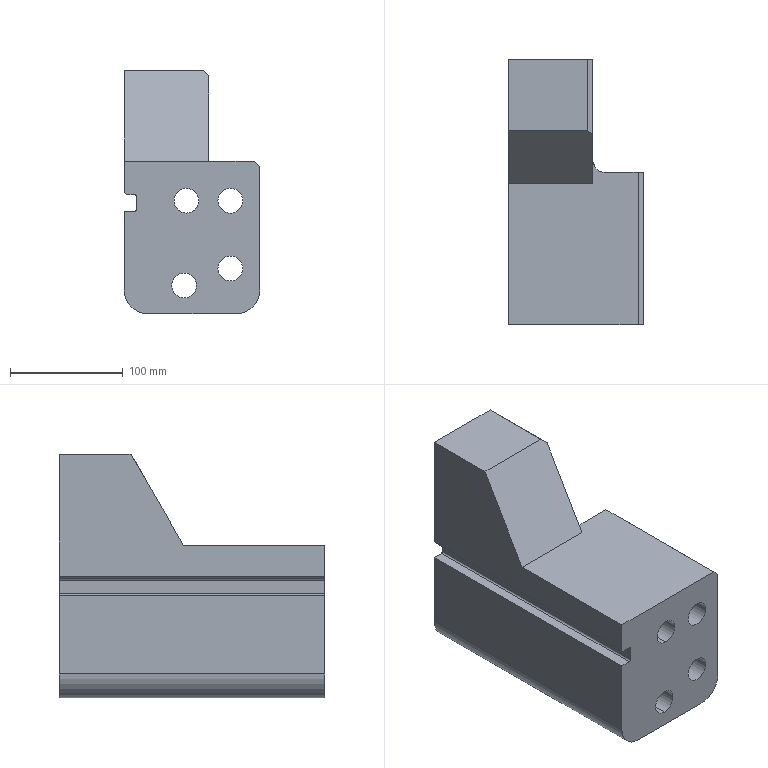Part | SolidWorks | features BaseBody 1 | 1 solid | 76 faces | box 120 x 235 x 215.5 mm | volume 3306577 mm3 | plane 35 | cylinder 31 | cone 8 | spline 2 | commonest cylinder face diameters 14 x8 22 x8 32 x8 20 x3 3 x2 42 x2